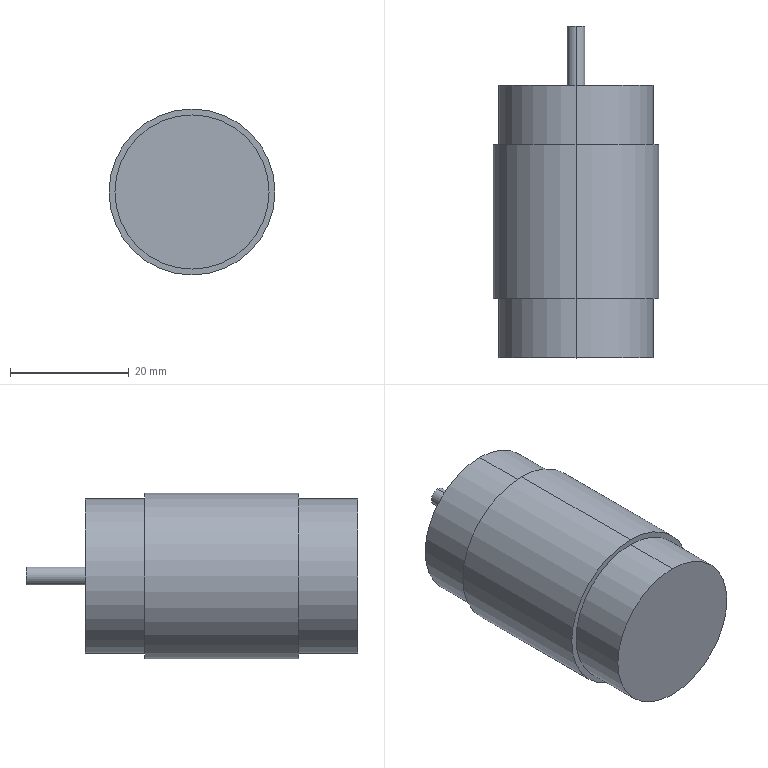Part | SolidWorks | features ICE 3, Extrusion 1 | 1 solid | 13 faces | box 28 x 56 x 28 mm | volume 26699 mm3 | cylinder 8 | plane 5 | commonest cylinder face diameters 26 x4 3 x2 28 x2
STEP:
#1=CARTESIAN_POINT('',(0.,56.,1.5));
#2=VERTEX_POINT('',#1);
#3=CARTESIAN_POINT('',(0.,56.,-1.5));
#4=VERTEX_POINT('',#3);
#5=CARTESIAN_POINT('',(0.,56.,0.));
#6=DIRECTION('',(0.,1.,0.));
#7=DIRECTION('',(0.,0.,1.));
#8=AXIS2_PLACEMENT_3D('',#5,#6,#7);
#9=CIRCLE('',#8,1.5);
#10=EDGE_CURVE('',#2,#4,#9,.T.);
#11=ORIENTED_EDGE('',*,*,#10,.F.);
#12=CARTESIAN_POINT('',(0.,46.,1.5));
#13=VERTEX_POINT('',#12);
#14=CARTESIAN_POINT('',(0.,56.,1.5));
#15=DIRECTION('',(0.,-1.,0.));
#16=VECTOR('',#15,1000.);
#17=LINE('',#14,#16);
#18=EDGE_CURVE('',#2,#13,#17,.T.);
#19=ORIENTED_EDGE('',*,*,#18,.T.);
#20=CARTESIAN_POINT('',(0.,46.,-1.5));
#21=VERTEX_POINT('',#20);
#22=CARTESIAN_POINT('',(0.,46.,0.));
#23=DIRECTION('',(0.,1.,0.));
#24=DIRECTION('',(0.,0.,1.));
#25=AXIS2_PLACEMENT_3D('',#22,#23,#24);
#26=CIRCLE('',#25,1.5);
#27=EDGE_CURVE('',#13,#21,#26,.T.);
#28=ORIENTED_EDGE('',*,*,#27,.T.);
#29=CARTESIAN_POINT('',(0.,56.,-1.5));
#30=DIRECTION('',(0.,-1.,0.));
#31=VECTOR('',#30,1000.);
#32=LINE('',#29,#31);
#33=EDGE_CURVE('',#4,#21,#32,.T.);
#34=ORIENTED_EDGE('',*,*,#33,.F.);
#35=EDGE_LOOP('',(#11,#19,#28,#34));
#36=FACE_OUTER_BOUND('',#35,.T.);
#37=CARTESIAN_POINT('',(0.,56.,0.));
#38=DIRECTION('',(0.,-1.,0.));
#39=DIRECTION('',(0.,0.,-1.));
#40=AXIS2_PLACEMENT_3D('',#37,#38,#39);
#41=CYLINDRICAL_SURFACE('',#40,1.5);
#42=ADVANCED_FACE('',(#36),#41,.T.);
#43=CARTESIAN_POINT('',(0.,46.,13.));
#44=VERTEX_POINT('',#43);
#45=CARTESIAN_POINT('',(0.,46.,-13.));
#46=VERTEX_POINT('',#45);
#47=CARTESIAN_POINT('',(0.,46.,0.));
#48=DIRECTION('',(0.,1.,0.));
#49=DIRECTION('',(0.,0.,1.));
#50=AXIS2_PLACEMENT_3D('',#47,#48,#49);
#51=CIRCLE('',#50,13.);
#52=EDGE_CURVE('',#44,#46,#51,.T.);
#53=ORIENTED_EDGE('',*,*,#52,.F.);
#54=CARTESIAN_POINT('',(0.,36.,13.));
#55=VERTEX_POINT('',#54);
#56=CARTESIAN_POINT('',(0.,46.,13.));
#57=DIRECTION('',(0.,-1.,0.));
#58=VECTOR('',#57,1000.);
#59=LINE('',#56,#58);
#60=EDGE_CURVE('',#44,#55,#59,.T.);
#61=ORIENTED_EDGE('',*,*,#60,.T.);
#62=CARTESIAN_POINT('',(0.,36.,-13.));
#63=VERTEX_POINT('',#62);
#64=CARTESIAN_POINT('',(0.,36.,0.));
#65=DIRECTION('',(0.,1.,0.));
#66=DIRECTION('',(0.,0.,1.));
#67=AXIS2_PLACEMENT_3D('',#64,#65,#66);
#68=CIRCLE('',#67,13.);
#69=EDGE_CURVE('',#55,#63,#68,.T.);
#70=ORIENTED_EDGE('',*,*,#69,.T.);
#71=CARTESIAN_POINT('',(0.,46.,-13.));
#72=DIRECTION('',(0.,-1.,0.));
#73=VECTOR('',#72,1000.);
#74=LINE('',#71,#73);
#75=EDGE_CURVE('',#46,#63,#74,.T.);
#76=ORIENTED_EDGE('',*,*,#75,.F.);
#77=EDGE_LOOP('',(#53,#61,#70,#76));
#78=FACE_OUTER_BOUND('',#77,.T.);
#79=CARTESIAN_POINT('',(0.,46.,0.));
#80=DIRECTION('',(0.,-1.,0.));
#81=DIRECTION('',(0.,0.,-1.));
#82=AXIS2_PLACEMENT_3D('',#79,#80,#81);
#83=CYLINDRICAL_SURFACE('',#82,13.);
#84=ADVANCED_FACE('',(#78),#83,.T.);
#85=CARTESIAN_POINT('',(0.,36.,14.));
#86=VERTEX_POINT('',#85);
#87=CARTESIAN_POINT('',(0.,36.,-14.));
#88=VERTEX_POINT('',#87);
#89=CARTESIAN_POINT('',(0.,36.,0.));
#90=DIRECTION('',(0.,1.,0.));
#91=DIRECTION('',(0.,0.,1.));
#92=AXIS2_PLACEMENT_3D('',#89,#90,#91);
#93=CIRCLE('',#92,14.);
#94=EDGE_CURVE('',#86,#88,#93,.T.);
#95=ORIENTED_EDGE('',*,*,#94,.F.);
#96=CARTESIAN_POINT('',(0.,10.,14.));
#97=VERTEX_POINT('',#96);
#98=CARTESIAN_POINT('',(0.,36.,14.));
#99=DIRECTION('',(0.,-1.,0.));
#100=VECTOR('',#99,1000.);
#101=LINE('',#98,#100);
#102=EDGE_CURVE('',#86,#97,#101,.T.);
#103=ORIENTED_EDGE('',*,*,#102,.T.);
#104=CARTESIAN_POINT('',(0.,10.,-14.));
#105=VERTEX_POINT('',#104);
#106=CARTESIAN_POINT('',(0.,10.,0.));
#107=DIRECTION('',(0.,1.,0.));
#108=DIRECTION('',(0.,0.,1.));
#109=AXIS2_PLACEMENT_3D('',#106,#107,#108);
#110=CIRCLE('',#109,14.);
#111=EDGE_CURVE('',#97,#105,#110,.T.);
#112=ORIENTED_EDGE('',*,*,#111,.T.);
#113=CARTESIAN_POINT('',(0.,36.,-14.));
#114=DIRECTION('',(0.,-1.,0.));
#115=VECTOR('',#114,1000.);
#116=LINE('',#113,#115);
#117=EDGE_CURVE('',#88,#105,#116,.T.);
#118=ORIENTED_EDGE('',*,*,#117,.F.);
#119=EDGE_LOOP('',(#95,#103,#112,#118));
#120=FACE_OUTER_BOUND('',#119,.T.);
#121=CARTESIAN_POINT('',(0.,36.,0.));
#122=DIRECTION('',(0.,-1.,0.));
#123=DIRECTION('',(0.,0.,-1.));
#124=AXIS2_PLACEMENT_3D('',#121,#122,#123);
#125=CYLINDRICAL_SURFACE('',#124,14.);
#126=ADVANCED_FACE('',(#120),#125,.T.);
#127=CARTESIAN_POINT('',(0.,10.,13.));
#128=VERTEX_POINT('',#127);
#129=CARTESIAN_POINT('',(0.,10.,-13.));
#130=VERTEX_POINT('',#129);
#131=CARTESIAN_POINT('',(0.,10.,0.));
#132=DIRECTION('',(0.,1.,0.));
#133=DIRECTION('',(0.,0.,1.));
#134=AXIS2_PLACEMENT_3D('',#131,#132,#133);
#135=CIRCLE('',#134,13.);
#136=EDGE_CURVE('',#128,#130,#135,.T.);
#137=ORIENTED_EDGE('',*,*,#136,.F.);
#138=CARTESIAN_POINT('',(0.,0.,13.));
#139=VERTEX_POINT('',#138);
#140=CARTESIAN_POINT('',(0.,10.,13.));
#141=DIRECTION('',(0.,-1.,0.));
#142=VECTOR('',#141,1000.);
#143=LINE('',#140,#142);
#144=EDGE_CURVE('',#128,#139,#143,.T.);
#145=ORIENTED_EDGE('',*,*,#144,.T.);
#146=CARTESIAN_POINT('',(0.,0.,-13.));
#147=VERTEX_POINT('',#146);
#148=CARTESIAN_POINT('',(0.,0.,0.));
#149=DIRECTION('',(0.,1.,0.));
#150=DIRECTION('',(0.,0.,1.));
#151=AXIS2_PLACEMENT_3D('',#148,#149,#150);
#152=CIRCLE('',#151,13.);
#153=EDGE_CURVE('',#139,#147,#152,.T.);
#154=ORIENTED_EDGE('',*,*,#153,.T.);
#155=CARTESIAN_POINT('',(0.,10.,-13.));
#156=DIRECTION('',(0.,-1.,0.));
#157=VECTOR('',#156,1000.);
#158=LINE('',#155,#157);
#159=EDGE_CURVE('',#130,#147,#158,.T.);
#160=ORIENTED_EDGE('',*,*,#159,.F.);
#161=EDGE_LOOP('',(#137,#145,#154,#160));
#162=FACE_OUTER_BOUND('',#161,.T.);
#163=CARTESIAN_POINT('',(0.,10.,0.));
#164=DIRECTION('',(0.,-1.,0.));
#165=DIRECTION('',(0.,0.,-1.));
#166=AXIS2_PLACEMENT_3D('',#163,#164,#165);
#167=CYLINDRICAL_SURFACE('',#166,13.);
#168=ADVANCED_FACE('',(#162),#167,.T.);
#169=ORIENTED_EDGE('',*,*,#144,.F.);
#170=CARTESIAN_POINT('',(0.,10.,0.));
#171=DIRECTION('',(0.,1.,0.));
#172=DIRECTION('',(0.,0.,1.));
#173=AXIS2_PLACEMENT_3D('',#170,#171,#172);
#174=CIRCLE('',#173,13.);
#175=EDGE_CURVE('',#130,#128,#174,.T.);
#176=ORIENTED_EDGE('',*,*,#175,.F.);
#177=ORIENTED_EDGE('',*,*,#159,.T.);
#178=CARTESIAN_POINT('',(0.,0.,0.));
#179=DIRECTION('',(0.,1.,0.));
#180=DIRECTION('',(0.,0.,1.));
#181=AXIS2_PLACEMENT_3D('',#178,#179,#180);
#182=CIRCLE('',#181,13.);
#183=EDGE_CURVE('',#147,#139,#182,.T.);
#184=ORIENTED_EDGE('',*,*,#183,.T.);
#185=EDGE_LOOP('',(#169,#176,#177,#184));
#186=FACE_OUTER_BOUND('',#185,.T.);
#187=CARTESIAN_POINT('',(0.,10.,0.));
#188=DIRECTION('',(0.,-1.,0.));
#189=DIRECTION('',(0.,0.,-1.));
#190=AXIS2_PLACEMENT_3D('',#187,#188,#189);
#191=CYLINDRICAL_SURFACE('',#190,13.);
#192=ADVANCED_FACE('',(#186),#191,.T.);
#193=ORIENTED_EDGE('',*,*,#183,.F.);
#194=ORIENTED_EDGE('',*,*,#153,.F.);
#195=EDGE_LOOP('',(#193,#194));
#196=FACE_OUTER_BOUND('',#195,.T.);
#197=CARTESIAN_POINT('',(0.,0.,0.));
#198=DIRECTION('',(0.,1.,0.));
#199=DIRECTION('',(0.,0.,1.));
#200=AXIS2_PLACEMENT_3D('',#197,#198,#199);
#201=PLANE('',#200);
#202=ADVANCED_FACE('',(#196),#201,.F.);
#203=ORIENTED_EDGE('',*,*,#102,.F.);
#204=CARTESIAN_POINT('',(0.,36.,0.));
#205=DIRECTION('',(0.,1.,0.));
#206=DIRECTION('',(0.,0.,1.));
#207=AXIS2_PLACEMENT_3D('',#204,#205,#206);
#208=CIRCLE('',#207,14.);
#209=EDGE_CURVE('',#88,#86,#208,.T.);
#210=ORIENTED_EDGE('',*,*,#209,.F.);
#211=ORIENTED_EDGE('',*,*,#117,.T.);
#212=CARTESIAN_POINT('',(0.,10.,0.));
#213=DIRECTION('',(0.,1.,0.));
#214=DIRECTION('',(0.,0.,1.));
#215=AXIS2_PLACEMENT_3D('',#212,#213,#214);
#216=CIRCLE('',#215,14.);
#217=EDGE_CURVE('',#105,#97,#216,.T.);
#218=ORIENTED_EDGE('',*,*,#217,.T.);
#219=EDGE_LOOP('',(#203,#210,#211,#218));
#220=FACE_OUTER_BOUND('',#219,.T.);
#221=CARTESIAN_POINT('',(0.,36.,0.));
#222=DIRECTION('',(0.,-1.,0.));
#223=DIRECTION('',(0.,0.,-1.));
#224=AXIS2_PLACEMENT_3D('',#221,#222,#223);
#225=CYLINDRICAL_SURFACE('',#224,14.);
#226=ADVANCED_FACE('',(#220),#225,.T.);
#227=CARTESIAN_POINT('',(0.,36.,0.));
#228=DIRECTION('',(0.,1.,0.));
#229=DIRECTION('',(0.,0.,1.));
#230=AXIS2_PLACEMENT_3D('',#227,#228,#229);
#231=CIRCLE('',#230,13.);
#232=EDGE_CURVE('',#63,#55,#231,.T.);
#233=ORIENTED_EDGE('',*,*,#232,.F.);
#234=ORIENTED_EDGE('',*,*,#69,.F.);
#235=EDGE_LOOP('',(#233,#234));
#236=FACE_BOUND('',#235,.T.);
#237=ORIENTED_EDGE('',*,*,#209,.T.);
#238=ORIENTED_EDGE('',*,*,#94,.T.);
#239=EDGE_LOOP('',(#237,#238));
#240=FACE_OUTER_BOUND('',#239,.T.);
#241=CARTESIAN_POINT('',(0.,36.,0.));
#242=DIRECTION('',(0.,1.,0.));
#243=DIRECTION('',(0.,0.,1.));
#244=AXIS2_PLACEMENT_3D('',#241,#242,#243);
#245=PLANE('',#244);
#246=ADVANCED_FACE('',(#236,#240),#245,.T.);
#247=ORIENTED_EDGE('',*,*,#175,.T.);
#248=ORIENTED_EDGE('',*,*,#136,.T.);
#249=EDGE_LOOP('',(#247,#248));
#250=FACE_BOUND('',#249,.T.);
#251=ORIENTED_EDGE('',*,*,#217,.F.);
#252=ORIENTED_EDGE('',*,*,#111,.F.);
#253=EDGE_LOOP('',(#251,#252));
#254=FACE_OUTER_BOUND('',#253,.T.);
#255=CARTESIAN_POINT('',(0.,10.,0.));
#256=DIRECTION('',(0.,1.,0.));
#257=DIRECTION('',(0.,0.,1.));
#258=AXIS2_PLACEMENT_3D('',#255,#256,#257);
#259=PLANE('',#258);
#260=ADVANCED_FACE('',(#250,#254),#259,.F.);
#261=ORIENTED_EDGE('',*,*,#60,.F.);
#262=CARTESIAN_POINT('',(0.,46.,0.));
#263=DIRECTION('',(0.,1.,0.));
#264=DIRECTION('',(0.,0.,1.));
#265=AXIS2_PLACEMENT_3D('',#262,#263,#264);
#266=CIRCLE('',#265,13.);
#267=EDGE_CURVE('',#46,#44,#266,.T.);
#268=ORIENTED_EDGE('',*,*,#267,.F.);
#269=ORIENTED_EDGE('',*,*,#75,.T.);
#270=ORIENTED_EDGE('',*,*,#232,.T.);
#271=EDGE_LOOP('',(#261,#268,#269,#270));
#272=FACE_OUTER_BOUND('',#271,.T.);
#273=CARTESIAN_POINT('',(0.,46.,0.));
#274=DIRECTION('',(0.,-1.,0.));
#275=DIRECTION('',(0.,0.,-1.));
#276=AXIS2_PLACEMENT_3D('',#273,#274,#275);
#277=CYLINDRICAL_SURFACE('',#276,13.);
#278=ADVANCED_FACE('',(#272),#277,.T.);
#279=CARTESIAN_POINT('',(0.,46.,0.));
#280=DIRECTION('',(0.,1.,0.));
#281=DIRECTION('',(0.,0.,1.));
#282=AXIS2_PLACEMENT_3D('',#279,#280,#281);
#283=CIRCLE('',#282,1.5);
#284=EDGE_CURVE('',#21,#13,#283,.T.);
#285=ORIENTED_EDGE('',*,*,#284,.F.);
#286=ORIENTED_EDGE('',*,*,#27,.F.);
#287=EDGE_LOOP('',(#285,#286));
#288=FACE_BOUND('',#287,.T.);
#289=ORIENTED_EDGE('',*,*,#267,.T.);
#290=ORIENTED_EDGE('',*,*,#52,.T.);
#291=EDGE_LOOP('',(#289,#290));
#292=FACE_OUTER_BOUND('',#291,.T.);
#293=CARTESIAN_POINT('',(0.,46.,0.));
#294=DIRECTION('',(0.,1.,0.));
#295=DIRECTION('',(0.,0.,1.));
#296=AXIS2_PLACEMENT_3D('',#293,#294,#295);
#297=PLANE('',#296);
#298=ADVANCED_FACE('',(#288,#292),#297,.T.);
#299=ORIENTED_EDGE('',*,*,#18,.F.);
#300=CARTESIAN_POINT('',(0.,56.,0.));
#301=DIRECTION('',(0.,1.,0.));
#302=DIRECTION('',(0.,0.,1.));
#303=AXIS2_PLACEMENT_3D('',#300,#301,#302);
#304=CIRCLE('',#303,1.5);
#305=EDGE_CURVE('',#4,#2,#304,.T.);
#306=ORIENTED_EDGE('',*,*,#305,.F.);
#307=ORIENTED_EDGE('',*,*,#33,.T.);
#308=ORIENTED_EDGE('',*,*,#284,.T.);
#309=EDGE_LOOP('',(#299,#306,#307,#308));
#310=FACE_OUTER_BOUND('',#309,.T.);
#311=CARTESIAN_POINT('',(0.,56.,0.));
#312=DIRECTION('',(0.,-1.,0.));
#313=DIRECTION('',(0.,0.,-1.));
#314=AXIS2_PLACEMENT_3D('',#311,#312,#313);
#315=CYLINDRICAL_SURFACE('',#314,1.5);
#316=ADVANCED_FACE('',(#310),#315,.T.);
#317=ORIENTED_EDGE('',*,*,#305,.T.);
#318=ORIENTED_EDGE('',*,*,#10,.T.);
#319=EDGE_LOOP('',(#317,#318));
#320=FACE_OUTER_BOUND('',#319,.T.);
#321=CARTESIAN_POINT('',(0.,56.,0.));
#322=DIRECTION('',(0.,1.,0.));
#323=DIRECTION('',(0.,0.,1.));
#324=AXIS2_PLACEMENT_3D('',#321,#322,#323);
#325=PLANE('',#324);
#326=ADVANCED_FACE('',(#320),#325,.T.);
#327=CLOSED_SHELL('',(#42,#84,#126,#168,#192,#202,#226,#246,#260,#278,#298,#316,#326));
#328=MANIFOLD_SOLID_BREP('',#327);
#329=CARTESIAN_POINT('',(0.,0.,0.));
#330=DIRECTION('',(0.,0.,1.));
#331=DIRECTION('',(1.,0.,0.));
#332=AXIS2_PLACEMENT_3D('',#329,#330,#331);
#333=(LENGTH_UNIT()NAMED_UNIT(*)SI_UNIT(.MILLI.,.METRE.));
#334=UNCERTAINTY_MEASURE_WITH_UNIT(LENGTH_MEASURE(0.00001),#333,'','');
#335=(NAMED_UNIT(*)PLANE_ANGLE_UNIT()SI_UNIT($,.RADIAN.));
#336=(NAMED_UNIT(*)SI_UNIT($,.STERADIAN.)SOLID_ANGLE_UNIT());
#337=(GEOMETRIC_REPRESENTATION_CONTEXT(3)GLOBAL_UNCERTAINTY_ASSIGNED_CONTEXT((#334))GLOBAL_UNIT_ASSIGNED_CONTEXT((#333,#335,#336))REPRESENTATION_CONTEXT('',''));
#338=ADVANCED_BREP_SHAPE_REPRESENTATION('',(#328,#332),#337);